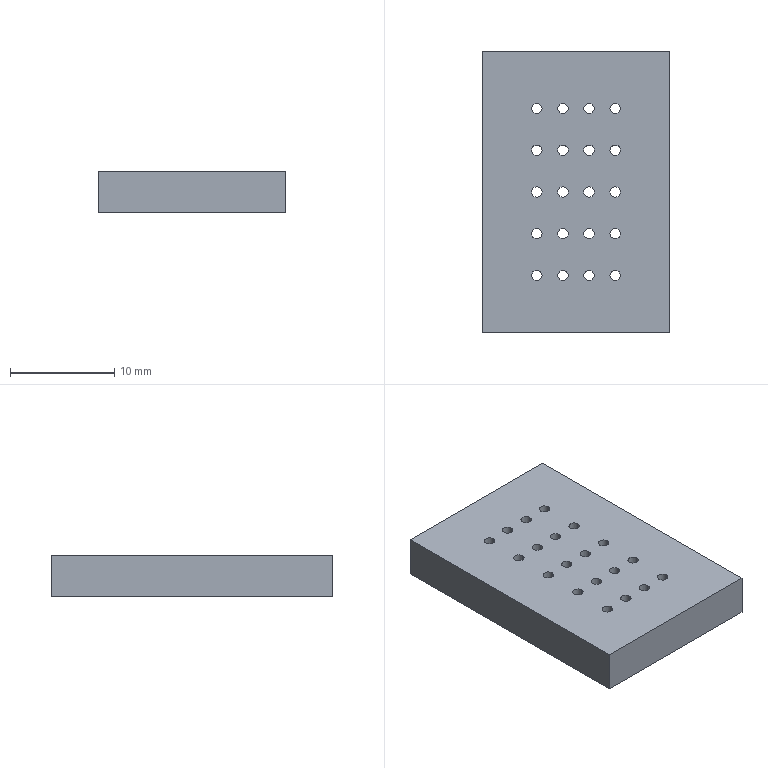Part | SolidWorks | features Extrusion 1, ICE 1, LPattern 1, MirrorPattern 1 | 1 solid | 46 faces | box 18 x 27 x 4 mm | volume 1881 mm3 | cylinder 40 | plane 6 | commonest cylinder face diameters 1 x40